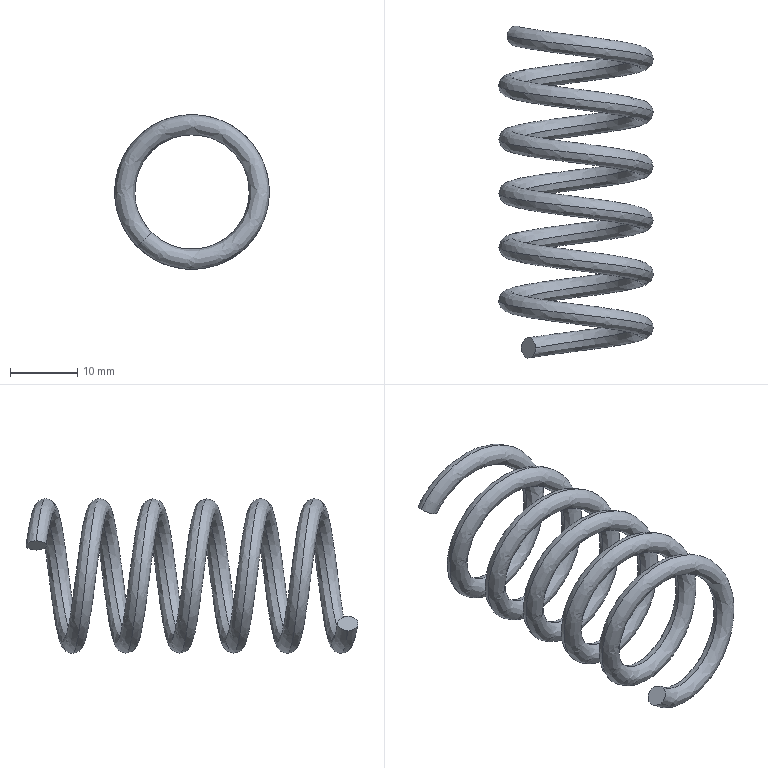Part | STEP file | Cuon T phu H01_16 | 1 solid | 4 faces | box 23 x 49.399 x 23 mm | volume 2577 mm3 | spline 2 | plane 2